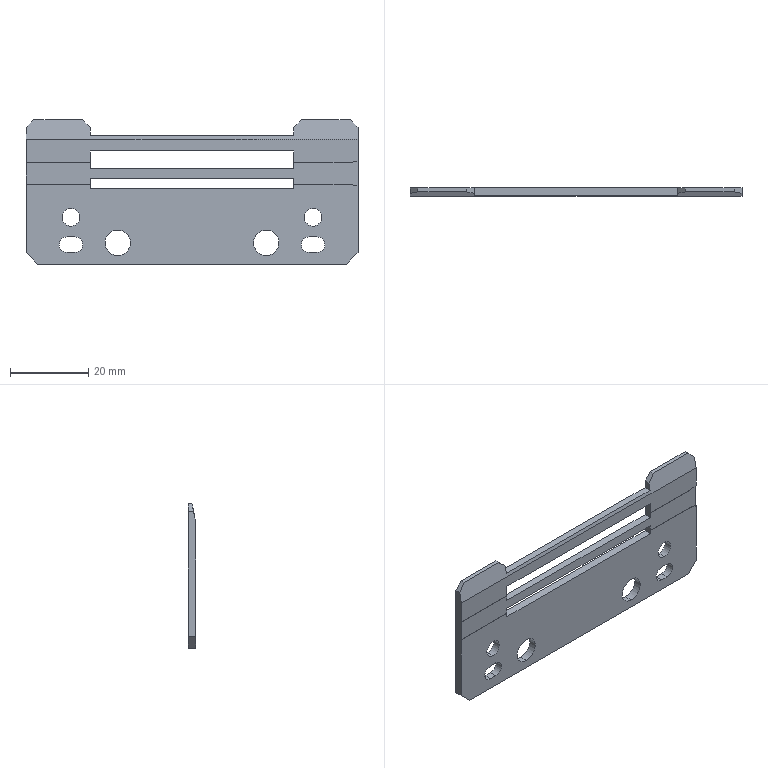Part | SolidWorks | features ICE 7, Chamfer 5, Cut 2, Extrusion 1 | 1 solid | 49 faces | box 85 x 2 x 37 mm | volume 4721 mm3 | plane 37 | cylinder 12 | commonest cylinder face diameters 4 x4 4.5 x4 6.5 x4